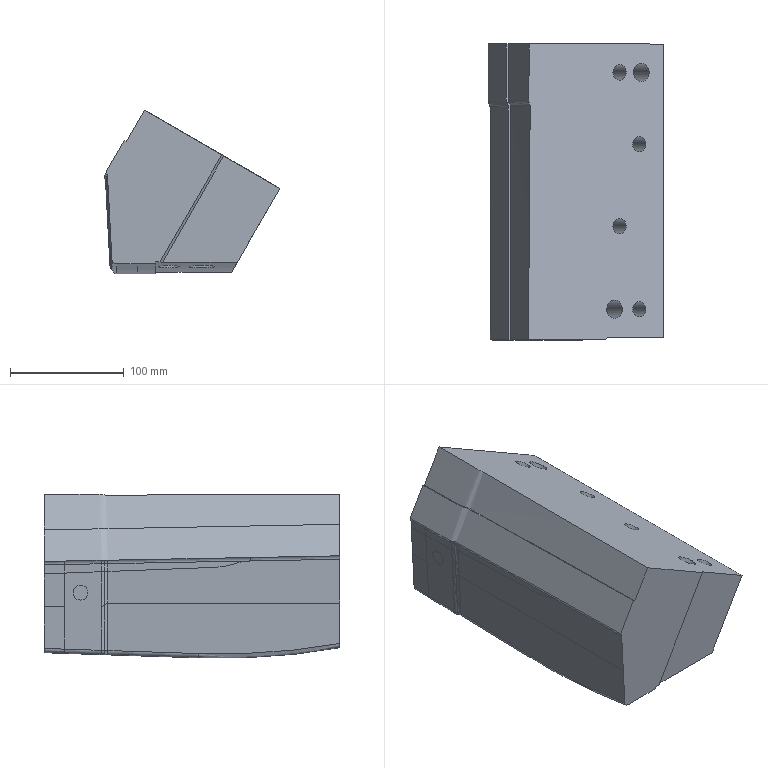Part | NX | features solid 2 | 1 solid | 56 faces | box 154.504 x 260 x 144.181 mm | volume 3650343 mm3 | spline 27 | plane 14 | cylinder 14 | sphere 1 | commonest cylinder face diameters 10 x4 13.5 x4 19.5 x4 16 x2